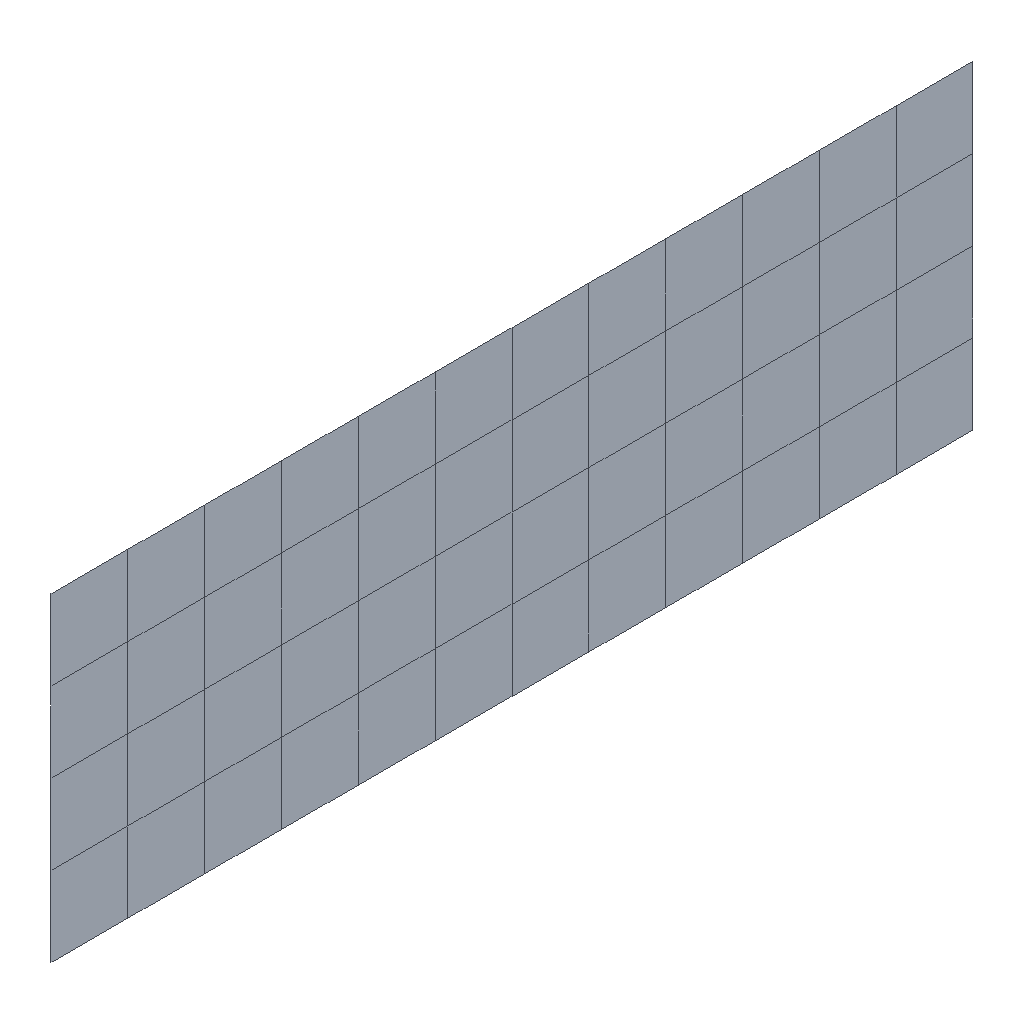Simulation study | abaqus
Set-up summary:
category,name,step,type,value,unit,region
solver,abaqus,,Abaqus/CAE 2024
units,SI m-kg-s (Pa),,inferred,E=3e+10 density=
analysis,Apply pressure,,static,time_period=1
mesh,nodes,,,177
mesh,elements,,,48
element_type,S8R5,,,48
material,Metal,,E,3e+10
material,Metal,,nu,0.3
load,Pressure,Apply pressure,pressure,20000,,_G7
bc,Fix,Apply pressure,encastre,[dofs=ENCASTRE],,EndA
bc,Rail,Apply pressure,fixed,"[dofs=rx,ry,rz,y,z n=5]",,EndB
Abaqus input file, long lists of numbers shortened:
*Heading
** Job name: deck Model name: Model-1
** Generated by: Abaqus/CAE 2024
*Preprint, echo=NO, model=NO, history=NO, contact=NO
**
** PARTS
**
*Part, name=Plate
*Node
      1,         -0.5, 0.08868,           0.
      2,         -0.5,  0.4887,           0.
** (175 more lines like these left out)
*Element, type=S8R5
 1,   1,   7,  36,  22,  66,  67,  68,  69
 2,   7,   8,  37,  36,  70,  71,  72,  67
** (46 more lines like these left out)
*Nset, nset=_G4, internal, generate
   1,  177,    1
*Elset, elset=_G4, internal, generate
  1,  48,   1
*Orientation, name=Ori-1
-0.866,         -0.5,           0.,         -0.5, 0.866,           0.
3, 0.
** Section: PlateSection
*Shell General Section, elset=_G4, material=Metal, orientation=Ori-1
0.008,
*End Part
**
**
** ASSEMBLY
**
*Assembly, name=Assembly
**
*Instance, name=Plate-1, part=Plate
*End Instance
**
*Nset, nset=EndA, instance=Plate-1
   3,   4,  15,  16,  17, 116, 119, 121, 123
*Elset, elset=EndA, instance=Plate-1, generate
 21,  24,   1
*Nset, nset=EndB, instance=Plate-1
   5,   6,  28,  29,  30, 170, 173, 175, 177
*Elset, elset=EndB, instance=Plate-1, generate
 45,  48,   1
*Nset, nset=MidSpan, instance=Plate-1
  1,  2,  7,  8,  9, 66, 70, 73, 76
*Elset, elset=MidSpan, instance=Plate-1
  1,  2,  3,  4, 25, 26, 27, 28
*Elset, elset=__G7_SPOS, internal, instance=Plate-1, generate
  1,  48,   1
*Surface, type=ELEMENT, name=_G7, internal
__G7_SPOS, SPOS
*Nset, nset="_T-Plate-1-Datum csys-1", internal
EndB,
*Transform, nset="_T-Plate-1-Datum csys-1"
-0.866,         -0.5,           0.,         -0.5, 0.866,           0.
*End Assembly
**
** MATERIALS
**
*Material, name=Metal
*Elastic
 3e+10, 0.3
** ----------------------------------------------------------------
**
** STEP: Apply pressure
**
*Step, name="Apply pressure", nlgeom=NO
Uniform pressure(20 kPa) load
*Static
1., 1., 1e-05, 1.
**
** BOUNDARY CONDITIONS
**
** Name: Fix left end Type: Symmetry/Antisymmetry/Encastre
*Boundary
EndA, ENCASTRE
** Name: Rail boundary condition Type: Displacement/Rotation
*Boundary
EndB, 2, 2
EndB, 3, 3
EndB, 4, 4
EndB, 5, 5
EndB, 6, 6
**
** LOADS
**
** Name: Pressure   Type: Pressure
*Dsload
_G7, P, 20000.
**
** OUTPUT REQUESTS
**
*Restart, write, frequency=0
**
** FIELD OUTPUT: F-Output-1
**
*Output, field
*Node Output
RF, U
*Element Output, directions=YES
E, S
**
** HISTORY OUTPUT: H-Output-1
**
*Output, history
*Node Output, nset=MidSpan
U3,
*End Step
Results summary:
result,odb.job_status,,,JOB_STATUS_COMPLETED_SUCCESSFULLY,"consistent, unstated (Abaqus has no unit system)"
result,steps[0].procedure,Apply pressure,,*STATIC,"consistent, unstated (Abaqus has no unit system)"
result,steps[0].time_period,Apply pressure,,1,"consistent, unstated (Abaqus has no unit system)"
result,steps[0].n_frames,Apply pressure,,2,"consistent, unstated (Abaqus has no unit system)"
result,steps[0].last_frame.id,Apply pressure,,1,"consistent, unstated (Abaqus has no unit system)"
result,steps[0].last_frame.value,Apply pressure,,1,"consistent, unstated (Abaqus has no unit system)"
result,steps[0].last_frame.description,Apply pressure,,Increment      1: Step Time =    1.000,"consistent, unstated (Abaqus has no unit system)"
result,steps[0].completed,Apply pressure,,True,"consistent, unstated (Abaqus has no unit system)"
result,steps[0].max_U_magnitude,Apply pressure,,0.05578,"consistent, unstated (Abaqus has no unit system)"
result,steps[0].max_S_mises,Apply pressure,,2.41893e+08,"consistent, unstated (Abaqus has no unit system)"
result,steps[0].RF_sum[1],Apply pressure,,0,"consistent, unstated (Abaqus has no unit system)"
result,steps[0].RF_sum[2],Apply pressure,,0,"consistent, unstated (Abaqus has no unit system)"
result,steps[0].RF_sum[3],Apply pressure,,8000,"consistent, unstated (Abaqus has no unit system)"